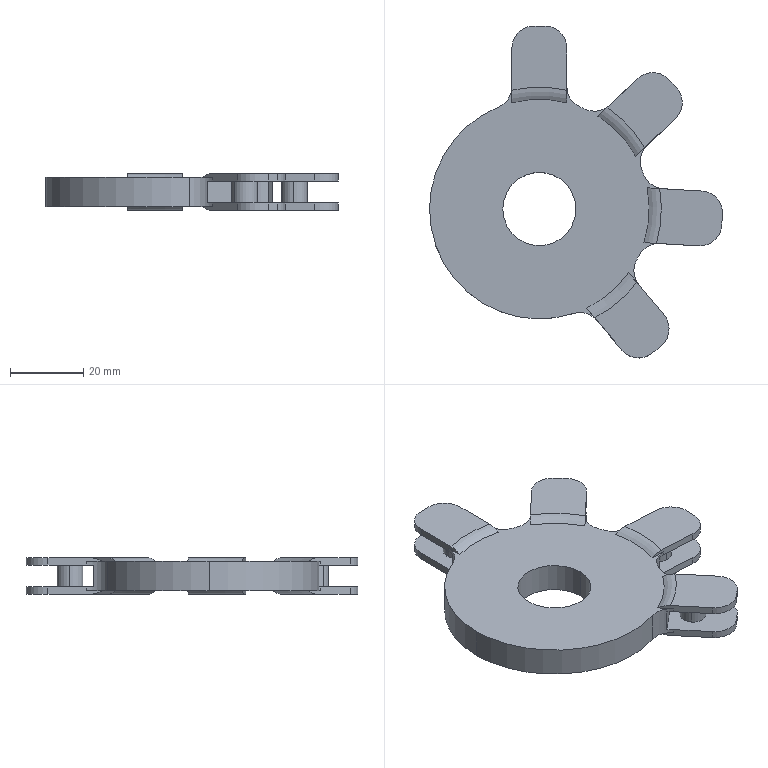Part | SolidWorks | features ICE 4, Fillet 2, CirPattern 1, Extrusion 1 | 1 solid | 93 faces | box 80.013 x 90.67 x 10 mm | volume 26380 mm3 | plane 46 | cylinder 39 | torus 8 | commonest cylinder face diameters 12 x24 7 x8 60 x5 20 x2